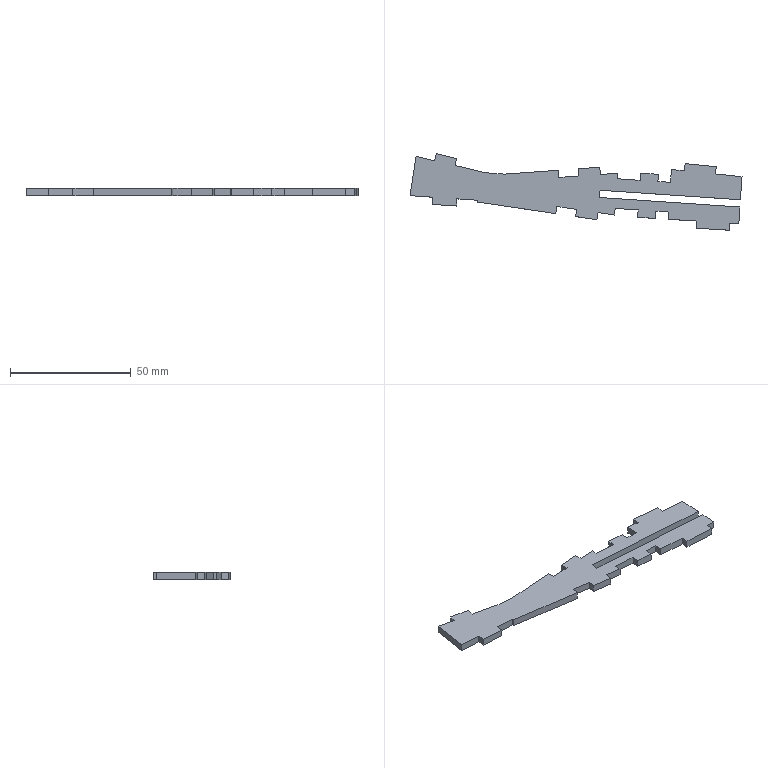Part | SolidWorks | features BaseBody 1 | 1 solid | 58 faces | box 137.742 x 31.731 x 3 mm | volume 6475 mm3 | plane 58